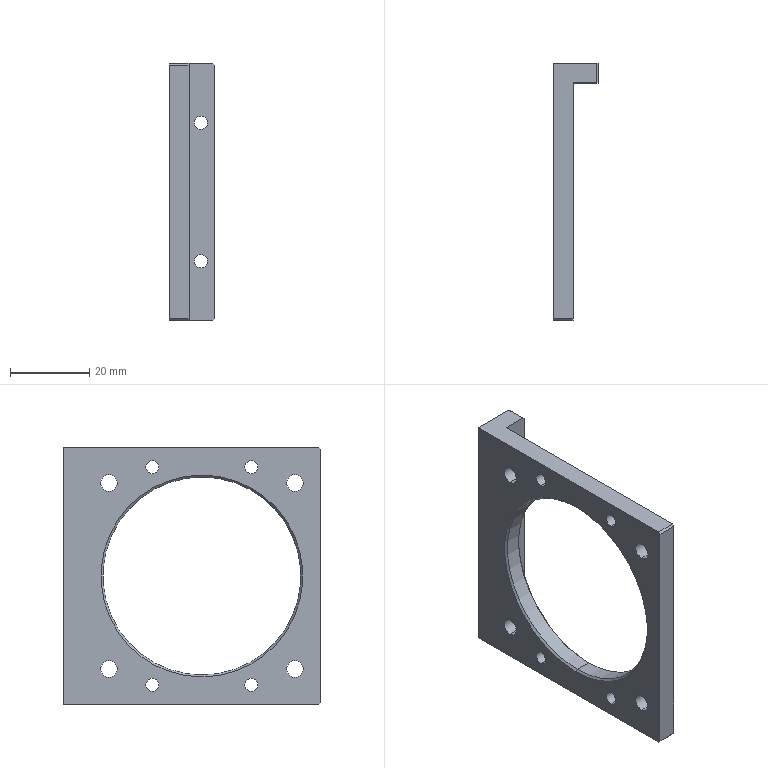Part | STEP file | Motor support plate | 1 solid | 38 faces | box 11.5 x 65 x 65 mm | volume 12844 mm3 | cylinder 22 | plane 12 | cone 4 | commonest cylinder face diameters 3.3 x12 4.2 x8 50 x2